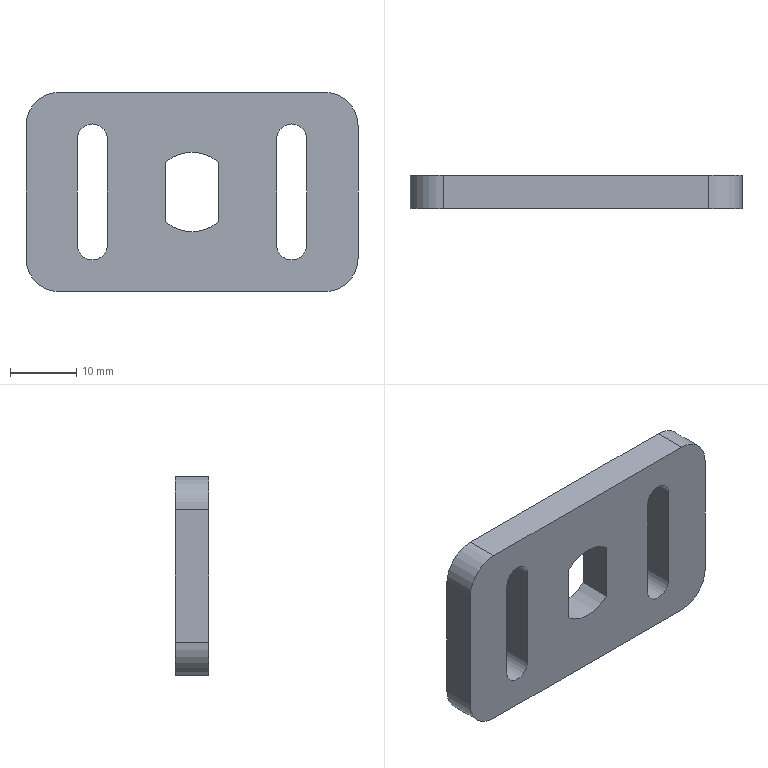Part | SolidWorks | features BaseBody 1 | 1 solid | 25 faces | box 50 x 5 x 30 mm | volume 6072 mm3 | cylinder 13 | plane 12 | commonest cylinder face diameters 4.5 x6 10 x4 12 x3
STEP:
#1=CARTESIAN_POINT('',(-12.75,0.,8.));
#2=VERTEX_POINT('',#1);
#3=CARTESIAN_POINT('',(-15.,0.,10.25));
#4=VERTEX_POINT('',#3);
#5=CARTESIAN_POINT('',(-15.,0.,8.));
#6=DIRECTION('',(0.,-1.,0.));
#7=DIRECTION('',(0.,0.,1.));
#8=AXIS2_PLACEMENT_3D('',#5,#6,#7);
#9=CIRCLE('',#8,2.25);
#10=EDGE_CURVE('',#2,#4,#9,.T.);
#11=ORIENTED_EDGE('',*,*,#10,.T.);
#12=CARTESIAN_POINT('',(-15.,5.,10.25));
#13=VERTEX_POINT('',#12);
#14=CARTESIAN_POINT('',(-15.,0.,10.25));
#15=DIRECTION('',(0.,1.,0.));
#16=VECTOR('',#15,1000.);
#17=LINE('',#14,#16);
#18=EDGE_CURVE('',#4,#13,#17,.T.);
#19=ORIENTED_EDGE('',*,*,#18,.T.);
#20=CARTESIAN_POINT('',(-12.75,5.,8.));
#21=VERTEX_POINT('',#20);
#22=CARTESIAN_POINT('',(-15.,5.,8.));
#23=DIRECTION('',(0.,-1.,0.));
#24=DIRECTION('',(0.,0.,1.));
#25=AXIS2_PLACEMENT_3D('',#22,#23,#24);
#26=CIRCLE('',#25,2.25);
#27=EDGE_CURVE('',#21,#13,#26,.T.);
#28=ORIENTED_EDGE('',*,*,#27,.F.);
#29=CARTESIAN_POINT('',(-12.75,0.,8.));
#30=DIRECTION('',(0.,-1.,0.));
#31=VECTOR('',#30,1000.);
#32=LINE('',#29,#31);
#33=EDGE_CURVE('',#21,#2,#32,.T.);
#34=ORIENTED_EDGE('',*,*,#33,.T.);
#35=EDGE_LOOP('',(#11,#19,#28,#34));
#36=FACE_OUTER_BOUND('',#35,.T.);
#37=CARTESIAN_POINT('',(-15.,0.,8.));
#38=DIRECTION('',(0.,1.,0.));
#39=DIRECTION('',(0.,0.,1.));
#40=AXIS2_PLACEMENT_3D('',#37,#38,#39);
#41=CYLINDRICAL_SURFACE('',#40,2.25);
#42=ADVANCED_FACE('',(#36),#41,.F.);
#43=CARTESIAN_POINT('',(17.25,0.,8.));
#44=VERTEX_POINT('',#43);
#45=CARTESIAN_POINT('',(15.,0.,10.25));
#46=VERTEX_POINT('',#45);
#47=CARTESIAN_POINT('',(15.,0.,8.));
#48=DIRECTION('',(0.,-1.,0.));
#49=DIRECTION('',(0.,0.,1.));
#50=AXIS2_PLACEMENT_3D('',#47,#48,#49);
#51=CIRCLE('',#50,2.25);
#52=EDGE_CURVE('',#44,#46,#51,.T.);
#53=ORIENTED_EDGE('',*,*,#52,.T.);
#54=CARTESIAN_POINT('',(15.,5.,10.25));
#55=VERTEX_POINT('',#54);
#56=CARTESIAN_POINT('',(15.,0.,10.25));
#57=DIRECTION('',(0.,1.,0.));
#58=VECTOR('',#57,1000.);
#59=LINE('',#56,#58);
#60=EDGE_CURVE('',#46,#55,#59,.T.);
#61=ORIENTED_EDGE('',*,*,#60,.T.);
#62=CARTESIAN_POINT('',(17.25,5.,8.));
#63=VERTEX_POINT('',#62);
#64=CARTESIAN_POINT('',(15.,5.,8.));
#65=DIRECTION('',(0.,-1.,0.));
#66=DIRECTION('',(0.,0.,1.));
#67=AXIS2_PLACEMENT_3D('',#64,#65,#66);
#68=CIRCLE('',#67,2.25);
#69=EDGE_CURVE('',#63,#55,#68,.T.);
#70=ORIENTED_EDGE('',*,*,#69,.F.);
#71=CARTESIAN_POINT('',(17.25,0.,8.));
#72=DIRECTION('',(0.,-1.,0.));
#73=VECTOR('',#72,1000.);
#74=LINE('',#71,#73);
#75=EDGE_CURVE('',#63,#44,#74,.T.);
#76=ORIENTED_EDGE('',*,*,#75,.T.);
#77=EDGE_LOOP('',(#53,#61,#70,#76));
#78=FACE_OUTER_BOUND('',#77,.T.);
#79=CARTESIAN_POINT('',(15.,0.,8.));
#80=DIRECTION('',(0.,1.,0.));
#81=DIRECTION('',(0.,0.,1.));
#82=AXIS2_PLACEMENT_3D('',#79,#80,#81);
#83=CYLINDRICAL_SURFACE('',#82,2.25);
#84=ADVANCED_FACE('',(#78),#83,.F.);
#85=CARTESIAN_POINT('',(4.,0.,4.472));
#86=VERTEX_POINT('',#85);
#87=CARTESIAN_POINT('',(0.,0.,6.));
#88=VERTEX_POINT('',#87);
#89=CARTESIAN_POINT('',(0.,0.,0.));
#90=DIRECTION('',(0.,-1.,0.));
#91=DIRECTION('',(0.,0.,1.));
#92=AXIS2_PLACEMENT_3D('',#89,#90,#91);
#93=CIRCLE('',#92,6.);
#94=EDGE_CURVE('',#86,#88,#93,.T.);
#95=ORIENTED_EDGE('',*,*,#94,.T.);
#96=CARTESIAN_POINT('',(0.,5.,6.));
#97=VERTEX_POINT('',#96);
#98=CARTESIAN_POINT('',(0.,0.,6.));
#99=DIRECTION('',(0.,1.,0.));
#100=VECTOR('',#99,1000.);
#101=LINE('',#98,#100);
#102=EDGE_CURVE('',#88,#97,#101,.T.);
#103=ORIENTED_EDGE('',*,*,#102,.T.);
#104=CARTESIAN_POINT('',(4.,5.,4.472));
#105=VERTEX_POINT('',#104);
#106=CARTESIAN_POINT('',(0.,5.,0.));
#107=DIRECTION('',(0.,-1.,0.));
#108=DIRECTION('',(0.,0.,1.));
#109=AXIS2_PLACEMENT_3D('',#106,#107,#108);
#110=CIRCLE('',#109,6.);
#111=EDGE_CURVE('',#105,#97,#110,.T.);
#112=ORIENTED_EDGE('',*,*,#111,.F.);
#113=CARTESIAN_POINT('',(4.,0.,4.472));
#114=DIRECTION('',(0.,-1.,0.));
#115=VECTOR('',#114,1000.);
#116=LINE('',#113,#115);
#117=EDGE_CURVE('',#105,#86,#116,.T.);
#118=ORIENTED_EDGE('',*,*,#117,.T.);
#119=EDGE_LOOP('',(#95,#103,#112,#118));
#120=FACE_OUTER_BOUND('',#119,.T.);
#121=CARTESIAN_POINT('',(0.,0.,0.));
#122=DIRECTION('',(0.,1.,0.));
#123=DIRECTION('',(0.,0.,1.));
#124=AXIS2_PLACEMENT_3D('',#121,#122,#123);
#125=CYLINDRICAL_SURFACE('',#124,6.);
#126=ADVANCED_FACE('',(#120),#125,.F.);
#127=CARTESIAN_POINT('',(25.,0.,-10.));
#128=VERTEX_POINT('',#127);
#129=CARTESIAN_POINT('',(20.,0.,-15.));
#130=VERTEX_POINT('',#129);
#131=CARTESIAN_POINT('',(20.,0.,-10.));
#132=DIRECTION('',(0.,1.,0.));
#133=DIRECTION('',(0.,0.,-1.));
#134=AXIS2_PLACEMENT_3D('',#131,#132,#133);
#135=CIRCLE('',#134,5.);
#136=EDGE_CURVE('',#128,#130,#135,.T.);
#137=ORIENTED_EDGE('',*,*,#136,.F.);
#138=CARTESIAN_POINT('',(25.,0.,10.));
#139=VERTEX_POINT('',#138);
#140=CARTESIAN_POINT('',(25.,0.,0.));
#141=DIRECTION('',(0.,0.,-1.));
#142=VECTOR('',#141,1000.);
#143=LINE('',#140,#142);
#144=EDGE_CURVE('',#139,#128,#143,.T.);
#145=ORIENTED_EDGE('',*,*,#144,.F.);
#146=CARTESIAN_POINT('',(20.,0.,15.));
#147=VERTEX_POINT('',#146);
#148=CARTESIAN_POINT('',(20.,0.,10.));
#149=DIRECTION('',(0.,1.,0.));
#150=DIRECTION('',(0.,0.,-1.));
#151=AXIS2_PLACEMENT_3D('',#148,#149,#150);
#152=CIRCLE('',#151,5.);
#153=EDGE_CURVE('',#147,#139,#152,.T.);
#154=ORIENTED_EDGE('',*,*,#153,.F.);
#155=CARTESIAN_POINT('',(-20.,0.,15.));
#156=VERTEX_POINT('',#155);
#157=CARTESIAN_POINT('',(0.,0.,15.));
#158=DIRECTION('',(1.,0.,0.));
#159=VECTOR('',#158,1000.);
#160=LINE('',#157,#159);
#161=EDGE_CURVE('',#156,#147,#160,.T.);
#162=ORIENTED_EDGE('',*,*,#161,.F.);
#163=CARTESIAN_POINT('',(-25.,0.,10.));
#164=VERTEX_POINT('',#163);
#165=CARTESIAN_POINT('',(-20.,0.,10.));
#166=DIRECTION('',(0.,1.,0.));
#167=DIRECTION('',(0.,0.,-1.));
#168=AXIS2_PLACEMENT_3D('',#165,#166,#167);
#169=CIRCLE('',#168,5.);
#170=EDGE_CURVE('',#164,#156,#169,.T.);
#171=ORIENTED_EDGE('',*,*,#170,.F.);
#172=CARTESIAN_POINT('',(-25.,0.,-10.));
#173=VERTEX_POINT('',#172);
#174=CARTESIAN_POINT('',(-25.,0.,0.));
#175=DIRECTION('',(0.,0.,1.));
#176=VECTOR('',#175,1000.);
#177=LINE('',#174,#176);
#178=EDGE_CURVE('',#173,#164,#177,.T.);
#179=ORIENTED_EDGE('',*,*,#178,.F.);
#180=CARTESIAN_POINT('',(-20.,0.,-15.));
#181=VERTEX_POINT('',#180);
#182=CARTESIAN_POINT('',(-20.,0.,-10.));
#183=DIRECTION('',(0.,1.,0.));
#184=DIRECTION('',(0.,0.,-1.));
#185=AXIS2_PLACEMENT_3D('',#182,#183,#184);
#186=CIRCLE('',#185,5.);
#187=EDGE_CURVE('',#181,#173,#186,.T.);
#188=ORIENTED_EDGE('',*,*,#187,.F.);
#189=CARTESIAN_POINT('',(0.,0.,-15.));
#190=DIRECTION('',(-1.,0.,0.));
#191=VECTOR('',#190,1000.);
#192=LINE('',#189,#191);
#193=EDGE_CURVE('',#130,#181,#192,.T.);
#194=ORIENTED_EDGE('',*,*,#193,.F.);
#195=EDGE_LOOP('',(#137,#145,#154,#162,#171,#179,#188,#194));
#196=FACE_OUTER_BOUND('',#195,.T.);
#197=CARTESIAN_POINT('',(-17.25,0.,-8.));
#198=VERTEX_POINT('',#197);
#199=CARTESIAN_POINT('',(-12.75,0.,-8.));
#200=VERTEX_POINT('',#199);
#201=CARTESIAN_POINT('',(-15.,0.,-8.));
#202=DIRECTION('',(0.,-1.,0.));
#203=DIRECTION('',(0.,0.,1.));
#204=AXIS2_PLACEMENT_3D('',#201,#202,#203);
#205=CIRCLE('',#204,2.25);
#206=EDGE_CURVE('',#198,#200,#205,.T.);
#207=ORIENTED_EDGE('',*,*,#206,.F.);
#208=CARTESIAN_POINT('',(-17.25,0.,8.));
#209=VERTEX_POINT('',#208);
#210=CARTESIAN_POINT('',(-17.25,0.,0.));
#211=DIRECTION('',(0.,0.,-1.));
#212=VECTOR('',#211,1000.);
#213=LINE('',#210,#212);
#214=EDGE_CURVE('',#209,#198,#213,.T.);
#215=ORIENTED_EDGE('',*,*,#214,.F.);
#216=CARTESIAN_POINT('',(-15.,0.,8.));
#217=DIRECTION('',(0.,-1.,0.));
#218=DIRECTION('',(0.,0.,1.));
#219=AXIS2_PLACEMENT_3D('',#216,#217,#218);
#220=CIRCLE('',#219,2.25);
#221=EDGE_CURVE('',#4,#209,#220,.T.);
#222=ORIENTED_EDGE('',*,*,#221,.F.);
#223=ORIENTED_EDGE('',*,*,#10,.F.);
#224=CARTESIAN_POINT('',(-12.75,0.,0.));
#225=DIRECTION('',(0.,0.,1.));
#226=VECTOR('',#225,1000.);
#227=LINE('',#224,#226);
#228=EDGE_CURVE('',#200,#2,#227,.T.);
#229=ORIENTED_EDGE('',*,*,#228,.F.);
#230=EDGE_LOOP('',(#207,#215,#222,#223,#229));
#231=FACE_BOUND('',#230,.T.);
#232=CARTESIAN_POINT('',(12.75,0.,-8.));
#233=VERTEX_POINT('',#232);
#234=CARTESIAN_POINT('',(17.25,0.,-8.));
#235=VERTEX_POINT('',#234);
#236=CARTESIAN_POINT('',(15.,0.,-8.));
#237=DIRECTION('',(0.,-1.,0.));
#238=DIRECTION('',(0.,0.,1.));
#239=AXIS2_PLACEMENT_3D('',#236,#237,#238);
#240=CIRCLE('',#239,2.25);
#241=EDGE_CURVE('',#233,#235,#240,.T.);
#242=ORIENTED_EDGE('',*,*,#241,.F.);
#243=CARTESIAN_POINT('',(12.75,0.,8.));
#244=VERTEX_POINT('',#243);
#245=CARTESIAN_POINT('',(12.75,0.,0.));
#246=DIRECTION('',(0.,0.,-1.));
#247=VECTOR('',#246,1000.);
#248=LINE('',#245,#247);
#249=EDGE_CURVE('',#244,#233,#248,.T.);
#250=ORIENTED_EDGE('',*,*,#249,.F.);
#251=CARTESIAN_POINT('',(15.,0.,8.));
#252=DIRECTION('',(0.,-1.,0.));
#253=DIRECTION('',(0.,0.,1.));
#254=AXIS2_PLACEMENT_3D('',#251,#252,#253);
#255=CIRCLE('',#254,2.25);
#256=EDGE_CURVE('',#46,#244,#255,.T.);
#257=ORIENTED_EDGE('',*,*,#256,.F.);
#258=ORIENTED_EDGE('',*,*,#52,.F.);
#259=CARTESIAN_POINT('',(17.25,0.,0.));
#260=DIRECTION('',(0.,0.,1.));
#261=VECTOR('',#260,1000.);
#262=LINE('',#259,#261);
#263=EDGE_CURVE('',#235,#44,#262,.T.);
#264=ORIENTED_EDGE('',*,*,#263,.F.);
#265=EDGE_LOOP('',(#242,#250,#257,#258,#264));
#266=FACE_BOUND('',#265,.T.);
#267=CARTESIAN_POINT('',(-4.,0.,-4.472));
#268=VERTEX_POINT('',#267);
#269=CARTESIAN_POINT('',(4.,0.,-4.472));
#270=VERTEX_POINT('',#269);
#271=CARTESIAN_POINT('',(0.,0.,0.));
#272=DIRECTION('',(0.,-1.,0.));
#273=DIRECTION('',(0.,0.,1.));
#274=AXIS2_PLACEMENT_3D('',#271,#272,#273);
#275=CIRCLE('',#274,6.);
#276=EDGE_CURVE('',#268,#270,#275,.T.);
#277=ORIENTED_EDGE('',*,*,#276,.F.);
#278=CARTESIAN_POINT('',(-4.,0.,4.472));
#279=VERTEX_POINT('',#278);
#280=CARTESIAN_POINT('',(-4.,0.,0.));
#281=DIRECTION('',(0.,0.,-1.));
#282=VECTOR('',#281,1000.);
#283=LINE('',#280,#282);
#284=EDGE_CURVE('',#279,#268,#283,.T.);
#285=ORIENTED_EDGE('',*,*,#284,.F.);
#286=CARTESIAN_POINT('',(0.,0.,0.));
#287=DIRECTION('',(0.,-1.,0.));
#288=DIRECTION('',(0.,0.,1.));
#289=AXIS2_PLACEMENT_3D('',#286,#287,#288);
#290=CIRCLE('',#289,6.);
#291=EDGE_CURVE('',#88,#279,#290,.T.);
#292=ORIENTED_EDGE('',*,*,#291,.F.);
#293=ORIENTED_EDGE('',*,*,#94,.F.);
#294=CARTESIAN_POINT('',(4.,0.,0.));
#295=DIRECTION('',(0.,0.,1.));
#296=VECTOR('',#295,1000.);
#297=LINE('',#294,#296);
#298=EDGE_CURVE('',#270,#86,#297,.T.);
#299=ORIENTED_EDGE('',*,*,#298,.F.);
#300=EDGE_LOOP('',(#277,#285,#292,#293,#299));
#301=FACE_BOUND('',#300,.T.);
#302=CARTESIAN_POINT('',(0.,0.,0.));
#303=DIRECTION('',(0.,1.,0.));
#304=DIRECTION('',(0.,0.,1.));
#305=AXIS2_PLACEMENT_3D('',#302,#303,#304);
#306=PLANE('',#305);
#307=ADVANCED_FACE('',(#196,#231,#266,#301),#306,.F.);
#308=CARTESIAN_POINT('',(20.,5.,-15.));
#309=VERTEX_POINT('',#308);
#310=CARTESIAN_POINT('',(20.,5.,-15.));
#311=DIRECTION('',(0.,1.,0.));
#312=VECTOR('',#311,1000.);
#313=LINE('',#310,#312);
#314=EDGE_CURVE('',#130,#309,#313,.T.);
#315=ORIENTED_EDGE('',*,*,#314,.F.);
#316=ORIENTED_EDGE('',*,*,#193,.T.);
#317=CARTESIAN_POINT('',(-20.,5.,-15.));
#318=VERTEX_POINT('',#317);
#319=CARTESIAN_POINT('',(-20.,5.,-15.));
#320=DIRECTION('',(0.,-1.,0.));
#321=VECTOR('',#320,1000.);
#322=LINE('',#319,#321);
#323=EDGE_CURVE('',#318,#181,#322,.T.);
#324=ORIENTED_EDGE('',*,*,#323,.F.);
#325=CARTESIAN_POINT('',(-25.,5.,-15.));
#326=DIRECTION('',(-1.,0.,0.));
#327=VECTOR('',#326,1000.);
#328=LINE('',#325,#327);
#329=EDGE_CURVE('',#309,#318,#328,.T.);
#330=ORIENTED_EDGE('',*,*,#329,.F.);
#331=EDGE_LOOP('',(#315,#316,#324,#330));
#332=FACE_OUTER_BOUND('',#331,.T.);
#333=CARTESIAN_POINT('',(-25.,5.,-15.));
#334=DIRECTION('',(0.,0.,1.));
#335=DIRECTION('',(1.,0.,0.));
#336=AXIS2_PLACEMENT_3D('',#333,#334,#335);
#337=PLANE('',#336);
#338=ADVANCED_FACE('',(#332),#337,.F.);
#339=ORIENTED_EDGE('',*,*,#136,.T.);
#340=ORIENTED_EDGE('',*,*,#314,.T.);
#341=CARTESIAN_POINT('',(25.,5.,-10.));
#342=VERTEX_POINT('',#341);
#343=CARTESIAN_POINT('',(20.,5.,-10.));
#344=DIRECTION('',(0.,-1.,0.));
#345=DIRECTION('',(0.,0.,-1.));
#346=AXIS2_PLACEMENT_3D('',#343,#344,#345);
#347=CIRCLE('',#346,5.);
#348=EDGE_CURVE('',#309,#342,#347,.T.);
#349=ORIENTED_EDGE('',*,*,#348,.T.);
#350=CARTESIAN_POINT('',(25.,5.,-10.));
#351=DIRECTION('',(0.,-1.,0.));
#352=VECTOR('',#351,1000.);
#353=LINE('',#350,#352);
#354=EDGE_CURVE('',#342,#128,#353,.T.);
#355=ORIENTED_EDGE('',*,*,#354,.T.);
#356=EDGE_LOOP('',(#339,#340,#349,#355));
#357=FACE_OUTER_BOUND('',#356,.T.);
#358=CARTESIAN_POINT('',(20.,5.,-10.));
#359=DIRECTION('',(0.,-1.,0.));
#360=DIRECTION('',(0.,0.,-1.));
#361=AXIS2_PLACEMENT_3D('',#358,#359,#360);
#362=CYLINDRICAL_SURFACE('',#361,5.);
#363=ADVANCED_FACE('',(#357),#362,.T.);
#364=ORIENTED_EDGE('',*,*,#354,.F.);
#365=CARTESIAN_POINT('',(25.,5.,10.));
#366=VERTEX_POINT('',#365);
#367=CARTESIAN_POINT('',(25.,5.,-15.));
#368=DIRECTION('',(0.,0.,-1.));
#369=VECTOR('',#368,1000.);
#370=LINE('',#367,#369);
#371=EDGE_CURVE('',#366,#342,#370,.T.);
#372=ORIENTED_EDGE('',*,*,#371,.F.);
#373=CARTESIAN_POINT('',(25.,5.,10.));
#374=DIRECTION('',(0.,1.,0.));
#375=VECTOR('',#374,1000.);
#376=LINE('',#373,#375);
#377=EDGE_CURVE('',#139,#366,#376,.T.);
#378=ORIENTED_EDGE('',*,*,#377,.F.);
#379=ORIENTED_EDGE('',*,*,#144,.T.);
#380=EDGE_LOOP('',(#364,#372,#378,#379));
#381=FACE_OUTER_BOUND('',#380,.T.);
#382=CARTESIAN_POINT('',(25.,5.,-15.));
#383=DIRECTION('',(-1.,0.,0.));
#384=DIRECTION('',(0.,0.,1.));
#385=AXIS2_PLACEMENT_3D('',#382,#383,#384);
#386=PLANE('',#385);
#387=ADVANCED_FACE('',(#381),#386,.F.);
#388=ORIENTED_EDGE('',*,*,#153,.T.);
#389=ORIENTED_EDGE('',*,*,#377,.T.);
#390=CARTESIAN_POINT('',(20.,5.,15.));
#391=VERTEX_POINT('',#390);
#392=CARTESIAN_POINT('',(20.,5.,10.));
#393=DIRECTION('',(0.,-1.,0.));
#394=DIRECTION('',(0.,0.,-1.));
#395=AXIS2_PLACEMENT_3D('',#392,#393,#394);
#396=CIRCLE('',#395,5.);
#397=EDGE_CURVE('',#366,#391,#396,.T.);
#398=ORIENTED_EDGE('',*,*,#397,.T.);
#399=CARTESIAN_POINT('',(20.,5.,15.));
#400=DIRECTION('',(0.,-1.,0.));
#401=VECTOR('',#400,1000.);
#402=LINE('',#399,#401);
#403=EDGE_CURVE('',#391,#147,#402,.T.);
#404=ORIENTED_EDGE('',*,*,#403,.T.);
#405=EDGE_LOOP('',(#388,#389,#398,#404));
#406=FACE_OUTER_BOUND('',#405,.T.);
#407=CARTESIAN_POINT('',(20.,5.,10.));
#408=DIRECTION('',(0.,-1.,0.));
#409=DIRECTION('',(0.,0.,-1.));
#410=AXIS2_PLACEMENT_3D('',#407,#408,#409);
#411=CYLINDRICAL_SURFACE('',#410,5.);
#412=ADVANCED_FACE('',(#406),#411,.T.);
#413=ORIENTED_EDGE('',*,*,#403,.F.);
#414=CARTESIAN_POINT('',(-20.,5.,15.));
#415=VERTEX_POINT('',#414);
#416=CARTESIAN_POINT('',(-25.,5.,15.));
#417=DIRECTION('',(1.,0.,0.));
#418=VECTOR('',#417,1000.);
#419=LINE('',#416,#418);
#420=EDGE_CURVE('',#415,#391,#419,.T.);
#421=ORIENTED_EDGE('',*,*,#420,.F.);
#422=CARTESIAN_POINT('',(-20.,5.,15.));
#423=DIRECTION('',(0.,1.,0.));
#424=VECTOR('',#423,1000.);
#425=LINE('',#422,#424);
#426=EDGE_CURVE('',#156,#415,#425,.T.);
#427=ORIENTED_EDGE('',*,*,#426,.F.);
#428=ORIENTED_EDGE('',*,*,#161,.T.);
#429=EDGE_LOOP('',(#413,#421,#427,#428));
#430=FACE_OUTER_BOUND('',#429,.T.);
#431=CARTESIAN_POINT('',(-25.,5.,15.));
#432=DIRECTION('',(0.,0.,-1.));
#433=DIRECTION('',(-1.,0.,0.));
#434=AXIS2_PLACEMENT_3D('',#431,#432,#433);
#435=PLANE('',#434);
#436=ADVANCED_FACE('',(#430),#435,.F.);
#437=ORIENTED_EDGE('',*,*,#170,.T.);
#438=ORIENTED_EDGE('',*,*,#426,.T.);
#439=CARTESIAN_POINT('',(-25.,5.,10.));
#440=VERTEX_POINT('',#439);
#441=CARTESIAN_POINT('',(-20.,5.,10.));
#442=DIRECTION('',(0.,-1.,0.));
#443=DIRECTION('',(0.,0.,-1.));
#444=AXIS2_PLACEMENT_3D('',#441,#442,#443);
#445=CIRCLE('',#444,5.);
#446=EDGE_CURVE('',#415,#440,#445,.T.);
#447=ORIENTED_EDGE('',*,*,#446,.T.);
#448=CARTESIAN_POINT('',(-25.,5.,10.));
#449=DIRECTION('',(0.,-1.,0.));
#450=VECTOR('',#449,1000.);
#451=LINE('',#448,#450);
#452=EDGE_CURVE('',#440,#164,#451,.T.);
#453=ORIENTED_EDGE('',*,*,#452,.T.);
#454=EDGE_LOOP('',(#437,#438,#447,#453));
#455=FACE_OUTER_BOUND('',#454,.T.);
#456=CARTESIAN_POINT('',(-20.,5.,10.));
#457=DIRECTION('',(0.,-1.,0.));
#458=DIRECTION('',(0.,0.,-1.));
#459=AXIS2_PLACEMENT_3D('',#456,#457,#458);
#460=CYLINDRICAL_SURFACE('',#459,5.);
#461=ADVANCED_FACE('',(#455),#460,.T.);
#462=ORIENTED_EDGE('',*,*,#452,.F.);
#463=CARTESIAN_POINT('',(-25.,5.,-10.));
#464=VERTEX_POINT('',#463);
#465=CARTESIAN_POINT('',(-25.,5.,-15.));
#466=DIRECTION('',(0.,0.,1.));
#467=VECTOR('',#466,1000.);
#468=LINE('',#465,#467);
#469=EDGE_CURVE('',#464,#440,#468,.T.);
#470=ORIENTED_EDGE('',*,*,#469,.F.);
#471=CARTESIAN_POINT('',(-25.,5.,-10.));
#472=DIRECTION('',(0.,1.,0.));
#473=VECTOR('',#472,1000.);
#474=LINE('',#471,#473);
#475=EDGE_CURVE('',#173,#464,#474,.T.);
#476=ORIENTED_EDGE('',*,*,#475,.F.);
#477=ORIENTED_EDGE('',*,*,#178,.T.);
#478=EDGE_LOOP('',(#462,#470,#476,#477));
#479=FACE_OUTER_BOUND('',#478,.T.);
#480=CARTESIAN_POINT('',(-25.,5.,-15.));
#481=DIRECTION('',(1.,0.,0.));
#482=DIRECTION('',(0.,0.,-1.));
#483=AXIS2_PLACEMENT_3D('',#480,#481,#482);
#484=PLANE('',#483);
#485=ADVANCED_FACE('',(#479),#484,.F.);
#486=ORIENTED_EDGE('',*,*,#187,.T.);
#487=ORIENTED_EDGE('',*,*,#475,.T.);
#488=CARTESIAN_POINT('',(-20.,5.,-10.));
#489=DIRECTION('',(0.,-1.,0.));
#490=DIRECTION('',(0.,0.,-1.));
#491=AXIS2_PLACEMENT_3D('',#488,#489,#490);
#492=CIRCLE('',#491,5.);
#493=EDGE_CURVE('',#464,#318,#492,.T.);
#494=ORIENTED_EDGE('',*,*,#493,.T.);
#495=ORIENTED_EDGE('',*,*,#323,.T.);
#496=EDGE_LOOP('',(#486,#487,#494,#495));
#497=FACE_OUTER_BOUND('',#496,.T.);
#498=CARTESIAN_POINT('',(-20.,5.,-10.));
#499=DIRECTION('',(0.,-1.,0.));
#500=DIRECTION('',(0.,0.,-1.));
#501=AXIS2_PLACEMENT_3D('',#498,#499,#500);
#502=CYLINDRICAL_SURFACE('',#501,5.);
#503=ADVANCED_FACE('',(#497),#502,.T.);
#504=CARTESIAN_POINT('',(-12.75,5.,-8.));
#505=VERTEX_POINT('',#504);
#506=CARTESIAN_POINT('',(-12.75,0.,-8.));
#507=DIRECTION('',(0.,1.,0.));
#508=VECTOR('',#507,1000.);
#509=LINE('',#506,#508);
#510=EDGE_CURVE('',#200,#505,#509,.T.);
#511=ORIENTED_EDGE('',*,*,#510,.F.);
#512=ORIENTED_EDGE('',*,*,#228,.T.);
#513=ORIENTED_EDGE('',*,*,#33,.F.);
#514=CARTESIAN_POINT('',(-12.75,5.,-8.));
#515=DIRECTION('',(0.,0.,1.));
#516=VECTOR('',#515,1000.);
#517=LINE('',#514,#516);
#518=EDGE_CURVE('',#505,#21,#517,.T.);
#519=ORIENTED_EDGE('',*,*,#518,.F.);
#520=EDGE_LOOP('',(#511,#512,#513,#519));
#521=FACE_OUTER_BOUND('',#520,.T.);
#522=CARTESIAN_POINT('',(-12.75,0.,-8.));
#523=DIRECTION('',(1.,0.,0.));
#524=DIRECTION('',(0.,0.,-1.));
#525=AXIS2_PLACEMENT_3D('',#522,#523,#524);
#526=PLANE('',#525);
#527=ADVANCED_FACE('',(#521),#526,.F.);
#528=CARTESIAN_POINT('',(-17.25,5.,-8.));
#529=VERTEX_POINT('',#528);
#530=CARTESIAN_POINT('',(-17.25,0.,-8.));
#531=DIRECTION('',(0.,1.,0.));
#532=VECTOR('',#531,1000.);
#533=LINE('',#530,#532);
#534=EDGE_CURVE('',#198,#529,#533,.T.);
#535=ORIENTED_EDGE('',*,*,#534,.F.);
#536=ORIENTED_EDGE('',*,*,#206,.T.);
#537=ORIENTED_EDGE('',*,*,#510,.T.);
#538=CARTESIAN_POINT('',(-15.,5.,-8.));
#539=DIRECTION('',(0.,-1.,0.));
#540=DIRECTION('',(0.,0.,1.));
#541=AXIS2_PLACEMENT_3D('',#538,#539,#540);
#542=CIRCLE('',#541,2.25);
#543=EDGE_CURVE('',#529,#505,#542,.T.);
#544=ORIENTED_EDGE('',*,*,#543,.F.);
#545=EDGE_LOOP('',(#535,#536,#537,#544));
#546=FACE_OUTER_BOUND('',#545,.T.);
#547=CARTESIAN_POINT('',(-15.,0.,-8.));
#548=DIRECTION('',(0.,1.,0.));
#549=DIRECTION('',(0.,0.,1.));
#550=AXIS2_PLACEMENT_3D('',#547,#548,#549);
#551=CYLINDRICAL_SURFACE('',#550,2.25);
#552=ADVANCED_FACE('',(#546),#551,.F.);
#553=CARTESIAN_POINT('',(-17.25,5.,8.));
#554=VERTEX_POINT('',#553);
#555=CARTESIAN_POINT('',(-17.25,0.,8.));
#556=DIRECTION('',(0.,1.,0.));
#557=VECTOR('',#556,1000.);
#558=LINE('',#555,#557);
#559=EDGE_CURVE('',#209,#554,#558,.T.);
#560=ORIENTED_EDGE('',*,*,#559,.F.);
#561=ORIENTED_EDGE('',*,*,#214,.T.);
#562=ORIENTED_EDGE('',*,*,#534,.T.);
#563=CARTESIAN_POINT('',(-17.25,5.,-8.));
#564=DIRECTION('',(0.,0.,-1.));
#565=VECTOR('',#564,1000.);
#566=LINE('',#563,#565);
#567=EDGE_CURVE('',#554,#529,#566,.T.);
#568=ORIENTED_EDGE('',*,*,#567,.F.);
#569=EDGE_LOOP('',(#560,#561,#562,#568));
#570=FACE_OUTER_BOUND('',#569,.T.);
#571=CARTESIAN_POINT('',(-17.25,0.,-8.));
#572=DIRECTION('',(-1.,0.,0.));
#573=DIRECTION('',(0.,0.,1.));
#574=AXIS2_PLACEMENT_3D('',#571,#572,#573);
#575=PLANE('',#574);
#576=ADVANCED_FACE('',(#570),#575,.F.);
#577=ORIENTED_EDGE('',*,*,#18,.F.);
#578=ORIENTED_EDGE('',*,*,#221,.T.);
#579=ORIENTED_EDGE('',*,*,#559,.T.);
#580=CARTESIAN_POINT('',(-15.,5.,8.));
#581=DIRECTION('',(0.,-1.,0.));
#582=DIRECTION('',(0.,0.,1.));
#583=AXIS2_PLACEMENT_3D('',#580,#581,#582);
#584=CIRCLE('',#583,2.25);
#585=EDGE_CURVE('',#13,#554,#584,.T.);
#586=ORIENTED_EDGE('',*,*,#585,.F.);
#587=EDGE_LOOP('',(#577,#578,#579,#586));
#588=FACE_OUTER_BOUND('',#587,.T.);
#589=CARTESIAN_POINT('',(-15.,0.,8.));
#590=DIRECTION('',(0.,1.,0.));
#591=DIRECTION('',(0.,0.,1.));
#592=AXIS2_PLACEMENT_3D('',#589,#590,#591);
#593=CYLINDRICAL_SURFACE('',#592,2.25);
#594=ADVANCED_FACE('',(#588),#593,.F.);
#595=CARTESIAN_POINT('',(17.25,5.,-8.));
#596=VERTEX_POINT('',#595);
#597=CARTESIAN_POINT('',(17.25,0.,-8.));
#598=DIRECTION('',(0.,1.,0.));
#599=VECTOR('',#598,1000.);
#600=LINE('',#597,#599);
#601=EDGE_CURVE('',#235,#596,#600,.T.);
#602=ORIENTED_EDGE('',*,*,#601,.F.);
#603=ORIENTED_EDGE('',*,*,#263,.T.);
#604=ORIENTED_EDGE('',*,*,#75,.F.);
#605=CARTESIAN_POINT('',(17.25,5.,-8.));
#606=DIRECTION('',(0.,0.,1.));
#607=VECTOR('',#606,1000.);
#608=LINE('',#605,#607);
#609=EDGE_CURVE('',#596,#63,#608,.T.);
#610=ORIENTED_EDGE('',*,*,#609,.F.);
#611=EDGE_LOOP('',(#602,#603,#604,#610));
#612=FACE_OUTER_BOUND('',#611,.T.);
#613=CARTESIAN_POINT('',(17.25,0.,-8.));
#614=DIRECTION('',(1.,0.,0.));
#615=DIRECTION('',(0.,0.,-1.));
#616=AXIS2_PLACEMENT_3D('',#613,#614,#615);
#617=PLANE('',#616);
#618=ADVANCED_FACE('',(#612),#617,.F.);
#619=CARTESIAN_POINT('',(12.75,5.,-8.));
#620=VERTEX_POINT('',#619);
#621=CARTESIAN_POINT('',(12.75,0.,-8.));
#622=DIRECTION('',(0.,1.,0.));
#623=VECTOR('',#622,1000.);
#624=LINE('',#621,#623);
#625=EDGE_CURVE('',#233,#620,#624,.T.);
#626=ORIENTED_EDGE('',*,*,#625,.F.);
#627=ORIENTED_EDGE('',*,*,#241,.T.);
#628=ORIENTED_EDGE('',*,*,#601,.T.);
#629=CARTESIAN_POINT('',(15.,5.,-8.));
#630=DIRECTION('',(0.,-1.,0.));
#631=DIRECTION('',(0.,0.,1.));
#632=AXIS2_PLACEMENT_3D('',#629,#630,#631);
#633=CIRCLE('',#632,2.25);
#634=EDGE_CURVE('',#620,#596,#633,.T.);
#635=ORIENTED_EDGE('',*,*,#634,.F.);
#636=EDGE_LOOP('',(#626,#627,#628,#635));
#637=FACE_OUTER_BOUND('',#636,.T.);
#638=CARTESIAN_POINT('',(15.,0.,-8.));
#639=DIRECTION('',(0.,1.,0.));
#640=DIRECTION('',(0.,0.,1.));
#641=AXIS2_PLACEMENT_3D('',#638,#639,#640);
#642=CYLINDRICAL_SURFACE('',#641,2.25);
#643=ADVANCED_FACE('',(#637),#642,.F.);
#644=CARTESIAN_POINT('',(12.75,5.,8.));
#645=VERTEX_POINT('',#644);
#646=CARTESIAN_POINT('',(12.75,0.,8.));
#647=DIRECTION('',(0.,1.,0.));
#648=VECTOR('',#647,1000.);
#649=LINE('',#646,#648);
#650=EDGE_CURVE('',#244,#645,#649,.T.);
#651=ORIENTED_EDGE('',*,*,#650,.F.);
#652=ORIENTED_EDGE('',*,*,#249,.T.);
#653=ORIENTED_EDGE('',*,*,#625,.T.);
#654=CARTESIAN_POINT('',(12.75,5.,-8.));
#655=DIRECTION('',(0.,0.,-1.));
#656=VECTOR('',#655,1000.);
#657=LINE('',#654,#656);
#658=EDGE_CURVE('',#645,#620,#657,.T.);
#659=ORIENTED_EDGE('',*,*,#658,.F.);
#660=EDGE_LOOP('',(#651,#652,#653,#659));
#661=FACE_OUTER_BOUND('',#660,.T.);
#662=CARTESIAN_POINT('',(12.75,0.,-8.));
#663=DIRECTION('',(-1.,0.,0.));
#664=DIRECTION('',(0.,0.,1.));
#665=AXIS2_PLACEMENT_3D('',#662,#663,#664);
#666=PLANE('',#665);
#667=ADVANCED_FACE('',(#661),#666,.F.);
#668=ORIENTED_EDGE('',*,*,#60,.F.);
#669=ORIENTED_EDGE('',*,*,#256,.T.);
#670=ORIENTED_EDGE('',*,*,#650,.T.);
#671=CARTESIAN_POINT('',(15.,5.,8.));
#672=DIRECTION('',(0.,-1.,0.));
#673=DIRECTION('',(0.,0.,1.));
#674=AXIS2_PLACEMENT_3D('',#671,#672,#673);
#675=CIRCLE('',#674,2.25);
#676=EDGE_CURVE('',#55,#645,#675,.T.);
#677=ORIENTED_EDGE('',*,*,#676,.F.);
#678=EDGE_LOOP('',(#668,#669,#670,#677));
#679=FACE_OUTER_BOUND('',#678,.T.);
#680=CARTESIAN_POINT('',(15.,0.,8.));
#681=DIRECTION('',(0.,1.,0.));
#682=DIRECTION('',(0.,0.,1.));
#683=AXIS2_PLACEMENT_3D('',#680,#681,#682);
#684=CYLINDRICAL_SURFACE('',#683,2.25);
#685=ADVANCED_FACE('',(#679),#684,.F.);
#686=CARTESIAN_POINT('',(4.,5.,-4.472));
#687=VERTEX_POINT('',#686);
#688=CARTESIAN_POINT('',(4.,0.,-4.472));
#689=DIRECTION('',(0.,1.,0.));
#690=VECTOR('',#689,1000.);
#691=LINE('',#688,#690);
#692=EDGE_CURVE('',#270,#687,#691,.T.);
#693=ORIENTED_EDGE('',*,*,#692,.F.);
#694=ORIENTED_EDGE('',*,*,#298,.T.);
#695=ORIENTED_EDGE('',*,*,#117,.F.);
#696=CARTESIAN_POINT('',(4.,5.,-4.472));
#697=DIRECTION('',(0.,0.,1.));
#698=VECTOR('',#697,1000.);
#699=LINE('',#696,#698);
#700=EDGE_CURVE('',#687,#105,#699,.T.);
#701=ORIENTED_EDGE('',*,*,#700,.F.);
#702=EDGE_LOOP('',(#693,#694,#695,#701));
#703=FACE_OUTER_BOUND('',#702,.T.);
#704=CARTESIAN_POINT('',(4.,0.,-4.472));
#705=DIRECTION('',(1.,0.,0.));
#706=DIRECTION('',(0.,0.,-1.));
#707=AXIS2_PLACEMENT_3D('',#704,#705,#706);
#708=PLANE('',#707);
#709=ADVANCED_FACE('',(#703),#708,.F.);
#710=CARTESIAN_POINT('',(-4.,5.,-4.472));
#711=VERTEX_POINT('',#710);
#712=CARTESIAN_POINT('',(-4.,0.,-4.472));
#713=DIRECTION('',(0.,1.,0.));
#714=VECTOR('',#713,1000.);
#715=LINE('',#712,#714);
#716=EDGE_CURVE('',#268,#711,#715,.T.);
#717=ORIENTED_EDGE('',*,*,#716,.F.);
#718=ORIENTED_EDGE('',*,*,#276,.T.);
#719=ORIENTED_EDGE('',*,*,#692,.T.);
#720=CARTESIAN_POINT('',(0.,5.,0.));
#721=DIRECTION('',(0.,-1.,0.));
#722=DIRECTION('',(0.,0.,1.));
#723=AXIS2_PLACEMENT_3D('',#720,#721,#722);
#724=CIRCLE('',#723,6.);
#725=EDGE_CURVE('',#711,#687,#724,.T.);
#726=ORIENTED_EDGE('',*,*,#725,.F.);
#727=EDGE_LOOP('',(#717,#718,#719,#726));
#728=FACE_OUTER_BOUND('',#727,.T.);
#729=CARTESIAN_POINT('',(0.,0.,0.));
#730=DIRECTION('',(0.,1.,0.));
#731=DIRECTION('',(0.,0.,1.));
#732=AXIS2_PLACEMENT_3D('',#729,#730,#731);
#733=CYLINDRICAL_SURFACE('',#732,6.);
#734=ADVANCED_FACE('',(#728),#733,.F.);
#735=CARTESIAN_POINT('',(-4.,5.,4.472));
#736=VERTEX_POINT('',#735);
#737=CARTESIAN_POINT('',(-4.,0.,4.472));
#738=DIRECTION('',(0.,1.,0.));
#739=VECTOR('',#738,1000.);
#740=LINE('',#737,#739);
#741=EDGE_CURVE('',#279,#736,#740,.T.);
#742=ORIENTED_EDGE('',*,*,#741,.F.);
#743=ORIENTED_EDGE('',*,*,#284,.T.);
#744=ORIENTED_EDGE('',*,*,#716,.T.);
#745=CARTESIAN_POINT('',(-4.,5.,-4.472));
#746=DIRECTION('',(0.,0.,-1.));
#747=VECTOR('',#746,1000.);
#748=LINE('',#745,#747);
#749=EDGE_CURVE('',#736,#711,#748,.T.);
#750=ORIENTED_EDGE('',*,*,#749,.F.);
#751=EDGE_LOOP('',(#742,#743,#744,#750));
#752=FACE_OUTER_BOUND('',#751,.T.);
#753=CARTESIAN_POINT('',(-4.,0.,-4.472));
#754=DIRECTION('',(-1.,0.,0.));
#755=DIRECTION('',(0.,0.,1.));
#756=AXIS2_PLACEMENT_3D('',#753,#754,#755);
#757=PLANE('',#756);
#758=ADVANCED_FACE('',(#752),#757,.F.);
#759=ORIENTED_EDGE('',*,*,#102,.F.);
#760=ORIENTED_EDGE('',*,*,#291,.T.);
#761=ORIENTED_EDGE('',*,*,#741,.T.);
#762=CARTESIAN_POINT('',(0.,5.,0.));
#763=DIRECTION('',(0.,-1.,0.));
#764=DIRECTION('',(0.,0.,1.));
#765=AXIS2_PLACEMENT_3D('',#762,#763,#764);
#766=CIRCLE('',#765,6.);
#767=EDGE_CURVE('',#97,#736,#766,.T.);
#768=ORIENTED_EDGE('',*,*,#767,.F.);
#769=EDGE_LOOP('',(#759,#760,#761,#768));
#770=FACE_OUTER_BOUND('',#769,.T.);
#771=CARTESIAN_POINT('',(0.,0.,0.));
#772=DIRECTION('',(0.,1.,0.));
#773=DIRECTION('',(0.,0.,1.));
#774=AXIS2_PLACEMENT_3D('',#771,#772,#773);
#775=CYLINDRICAL_SURFACE('',#774,6.);
#776=ADVANCED_FACE('',(#770),#775,.F.);
#777=ORIENTED_EDGE('',*,*,#420,.T.);
#778=ORIENTED_EDGE('',*,*,#397,.F.);
#779=ORIENTED_EDGE('',*,*,#371,.T.);
#780=ORIENTED_EDGE('',*,*,#348,.F.);
#781=ORIENTED_EDGE('',*,*,#329,.T.);
#782=ORIENTED_EDGE('',*,*,#493,.F.);
#783=ORIENTED_EDGE('',*,*,#469,.T.);
#784=ORIENTED_EDGE('',*,*,#446,.F.);
#785=EDGE_LOOP('',(#777,#778,#779,#780,#781,#782,#783,#784));
#786=FACE_OUTER_BOUND('',#785,.T.);
#787=ORIENTED_EDGE('',*,*,#27,.T.);
#788=ORIENTED_EDGE('',*,*,#585,.T.);
#789=ORIENTED_EDGE('',*,*,#567,.T.);
#790=ORIENTED_EDGE('',*,*,#543,.T.);
#791=ORIENTED_EDGE('',*,*,#518,.T.);
#792=EDGE_LOOP('',(#787,#788,#789,#790,#791));
#793=FACE_BOUND('',#792,.T.);
#794=ORIENTED_EDGE('',*,*,#69,.T.);
#795=ORIENTED_EDGE('',*,*,#676,.T.);
#796=ORIENTED_EDGE('',*,*,#658,.T.);
#797=ORIENTED_EDGE('',*,*,#634,.T.);
#798=ORIENTED_EDGE('',*,*,#609,.T.);
#799=EDGE_LOOP('',(#794,#795,#796,#797,#798));
#800=FACE_BOUND('',#799,.T.);
#801=ORIENTED_EDGE('',*,*,#111,.T.);
#802=ORIENTED_EDGE('',*,*,#767,.T.);
#803=ORIENTED_EDGE('',*,*,#749,.T.);
#804=ORIENTED_EDGE('',*,*,#725,.T.);
#805=ORIENTED_EDGE('',*,*,#700,.T.);
#806=EDGE_LOOP('',(#801,#802,#803,#804,#805));
#807=FACE_BOUND('',#806,.T.);
#808=CARTESIAN_POINT('',(0.,5.,0.));
#809=DIRECTION('',(0.,1.,0.));
#810=DIRECTION('',(0.,0.,1.));
#811=AXIS2_PLACEMENT_3D('',#808,#809,#810);
#812=PLANE('',#811);
#813=ADVANCED_FACE('',(#786,#793,#800,#807),#812,.T.);
#814=CLOSED_SHELL('',(#42,#84,#126,#307,#338,#363,#387,#412,#436,#461,#485,#503,#527,#552,#576,#594,#618,#643,#667,#685,#709,#734,#758,#776,#813));
#815=MANIFOLD_SOLID_BREP('',#814);
#816=CARTESIAN_POINT('',(0.,0.,0.));
#817=DIRECTION('',(0.,0.,1.));
#818=DIRECTION('',(1.,0.,0.));
#819=AXIS2_PLACEMENT_3D('',#816,#817,#818);
#820=(LENGTH_UNIT()NAMED_UNIT(*)SI_UNIT(.MILLI.,.METRE.));
#821=UNCERTAINTY_MEASURE_WITH_UNIT(LENGTH_MEASURE(0.00001),#820,'','');
#822=(NAMED_UNIT(*)PLANE_ANGLE_UNIT()SI_UNIT($,.RADIAN.));
#823=(NAMED_UNIT(*)SI_UNIT($,.STERADIAN.)SOLID_ANGLE_UNIT());
#824=(GEOMETRIC_REPRESENTATION_CONTEXT(3)GLOBAL_UNCERTAINTY_ASSIGNED_CONTEXT((#821))GLOBAL_UNIT_ASSIGNED_CONTEXT((#820,#822,#823))REPRESENTATION_CONTEXT('',''));
#825=ADVANCED_BREP_SHAPE_REPRESENTATION('',(#815,#819),#824);